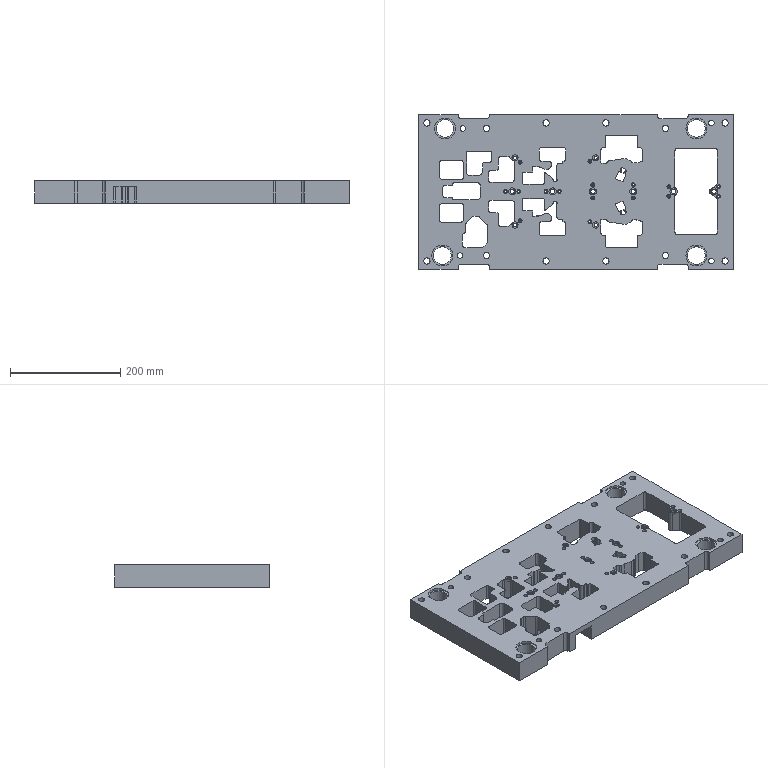Part | NX | features PS-1 2 | 1 solid | 585 faces | box 570 x 280 x 40 mm | volume 4455388 mm3 | plane 277 | cylinder 262 | spline 46 | commonest cylinder face diameters 8 x57 6 x32 10 x18 4.001 x16 7 x16 11 x15